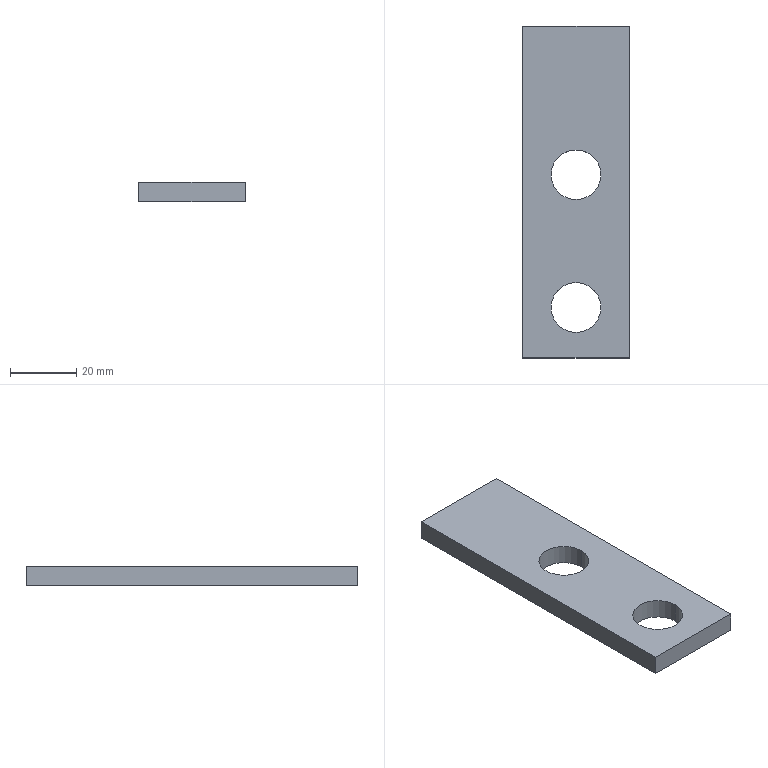Part | SolidWorks | features FlatPattern 1, SMBaseFlange 1, SheetMetal 1 | 1 solid | 10 faces | box 32 x 100 x 6 mm | volume 17079 mm3 | plane 6 | cylinder 4 | commonest cylinder face diameters 15 x4
STEP:
#1=CARTESIAN_POINT('',(8.5,-84.8,-6.));
#2=VERTEX_POINT('',#1);
#3=CARTESIAN_POINT('',(23.5,-84.8,-6.));
#4=VERTEX_POINT('',#3);
#5=CARTESIAN_POINT('',(16.,-84.8,-6.));
#6=DIRECTION('',(0.,0.,1.));
#7=DIRECTION('',(1.,0.,0.));
#8=AXIS2_PLACEMENT_3D('',#5,#6,#7);
#9=CIRCLE('',#8,7.5);
#10=EDGE_CURVE('',#2,#4,#9,.T.);
#11=ORIENTED_EDGE('',*,*,#10,.F.);
#12=CARTESIAN_POINT('',(8.5,-84.8,0.));
#13=VERTEX_POINT('',#12);
#14=CARTESIAN_POINT('',(8.5,-84.8,-6.));
#15=DIRECTION('',(0.,0.,1.));
#16=VECTOR('',#15,1000.);
#17=LINE('',#14,#16);
#18=EDGE_CURVE('',#2,#13,#17,.T.);
#19=ORIENTED_EDGE('',*,*,#18,.T.);
#20=CARTESIAN_POINT('',(23.5,-84.8,0.));
#21=VERTEX_POINT('',#20);
#22=CARTESIAN_POINT('',(16.,-84.8,0.));
#23=DIRECTION('',(0.,0.,1.));
#24=DIRECTION('',(1.,0.,0.));
#25=AXIS2_PLACEMENT_3D('',#22,#23,#24);
#26=CIRCLE('',#25,7.5);
#27=EDGE_CURVE('',#13,#21,#26,.T.);
#28=ORIENTED_EDGE('',*,*,#27,.T.);
#29=CARTESIAN_POINT('',(23.5,-84.8,-6.));
#30=DIRECTION('',(0.,0.,1.));
#31=VECTOR('',#30,1000.);
#32=LINE('',#29,#31);
#33=EDGE_CURVE('',#4,#21,#32,.T.);
#34=ORIENTED_EDGE('',*,*,#33,.F.);
#35=EDGE_LOOP('',(#11,#19,#28,#34));
#36=FACE_OUTER_BOUND('',#35,.T.);
#37=CARTESIAN_POINT('',(16.,-84.8,-6.));
#38=DIRECTION('',(0.,0.,1.));
#39=DIRECTION('',(1.,0.,0.));
#40=AXIS2_PLACEMENT_3D('',#37,#38,#39);
#41=CYLINDRICAL_SURFACE('',#40,7.5);
#42=ADVANCED_FACE('',(#36),#41,.F.);
#43=CARTESIAN_POINT('',(8.5,-44.8,-6.));
#44=VERTEX_POINT('',#43);
#45=CARTESIAN_POINT('',(23.5,-44.8,-6.));
#46=VERTEX_POINT('',#45);
#47=CARTESIAN_POINT('',(16.,-44.8,-6.));
#48=DIRECTION('',(0.,0.,1.));
#49=DIRECTION('',(1.,0.,0.));
#50=AXIS2_PLACEMENT_3D('',#47,#48,#49);
#51=CIRCLE('',#50,7.5);
#52=EDGE_CURVE('',#44,#46,#51,.T.);
#53=ORIENTED_EDGE('',*,*,#52,.F.);
#54=CARTESIAN_POINT('',(8.5,-44.8,0.));
#55=VERTEX_POINT('',#54);
#56=CARTESIAN_POINT('',(8.5,-44.8,-6.));
#57=DIRECTION('',(0.,0.,1.));
#58=VECTOR('',#57,1000.);
#59=LINE('',#56,#58);
#60=EDGE_CURVE('',#44,#55,#59,.T.);
#61=ORIENTED_EDGE('',*,*,#60,.T.);
#62=CARTESIAN_POINT('',(23.5,-44.8,0.));
#63=VERTEX_POINT('',#62);
#64=CARTESIAN_POINT('',(16.,-44.8,0.));
#65=DIRECTION('',(0.,0.,1.));
#66=DIRECTION('',(1.,0.,0.));
#67=AXIS2_PLACEMENT_3D('',#64,#65,#66);
#68=CIRCLE('',#67,7.5);
#69=EDGE_CURVE('',#55,#63,#68,.T.);
#70=ORIENTED_EDGE('',*,*,#69,.T.);
#71=CARTESIAN_POINT('',(23.5,-44.8,-6.));
#72=DIRECTION('',(0.,0.,1.));
#73=VECTOR('',#72,1000.);
#74=LINE('',#71,#73);
#75=EDGE_CURVE('',#46,#63,#74,.T.);
#76=ORIENTED_EDGE('',*,*,#75,.F.);
#77=EDGE_LOOP('',(#53,#61,#70,#76));
#78=FACE_OUTER_BOUND('',#77,.T.);
#79=CARTESIAN_POINT('',(16.,-44.8,-6.));
#80=DIRECTION('',(0.,0.,1.));
#81=DIRECTION('',(1.,0.,0.));
#82=AXIS2_PLACEMENT_3D('',#79,#80,#81);
#83=CYLINDRICAL_SURFACE('',#82,7.5);
#84=ADVANCED_FACE('',(#78),#83,.F.);
#85=CARTESIAN_POINT('',(0.,0.,0.));
#86=VERTEX_POINT('',#85);
#87=CARTESIAN_POINT('',(0.,-100.,0.));
#88=VERTEX_POINT('',#87);
#89=CARTESIAN_POINT('',(0.,0.,0.));
#90=DIRECTION('',(0.,-1.,0.));
#91=VECTOR('',#90,1000.);
#92=LINE('',#89,#91);
#93=EDGE_CURVE('',#86,#88,#92,.T.);
#94=ORIENTED_EDGE('',*,*,#93,.F.);
#95=CARTESIAN_POINT('',(0.,0.,-6.));
#96=VERTEX_POINT('',#95);
#97=CARTESIAN_POINT('',(0.,0.,-6.));
#98=DIRECTION('',(0.,0.,1.));
#99=VECTOR('',#98,1000.);
#100=LINE('',#97,#99);
#101=EDGE_CURVE('',#96,#86,#100,.T.);
#102=ORIENTED_EDGE('',*,*,#101,.F.);
#103=CARTESIAN_POINT('',(0.,-100.,-6.));
#104=VERTEX_POINT('',#103);
#105=CARTESIAN_POINT('',(0.,0.,-6.));
#106=DIRECTION('',(0.,-1.,0.));
#107=VECTOR('',#106,1000.);
#108=LINE('',#105,#107);
#109=EDGE_CURVE('',#96,#104,#108,.T.);
#110=ORIENTED_EDGE('',*,*,#109,.T.);
#111=CARTESIAN_POINT('',(0.,-100.,-6.));
#112=DIRECTION('',(0.,0.,1.));
#113=VECTOR('',#112,1000.);
#114=LINE('',#111,#113);
#115=EDGE_CURVE('',#104,#88,#114,.T.);
#116=ORIENTED_EDGE('',*,*,#115,.T.);
#117=EDGE_LOOP('',(#94,#102,#110,#116));
#118=FACE_OUTER_BOUND('',#117,.T.);
#119=CARTESIAN_POINT('',(0.,0.,-6.));
#120=DIRECTION('',(-1.,0.,0.));
#121=DIRECTION('',(0.,-1.,0.));
#122=AXIS2_PLACEMENT_3D('',#119,#120,#121);
#123=PLANE('',#122);
#124=ADVANCED_FACE('',(#118),#123,.T.);
#125=CARTESIAN_POINT('',(32.,0.,0.));
#126=VERTEX_POINT('',#125);
#127=CARTESIAN_POINT('',(0.,0.,0.));
#128=DIRECTION('',(-1.,0.,0.));
#129=VECTOR('',#128,1000.);
#130=LINE('',#127,#129);
#131=EDGE_CURVE('',#126,#86,#130,.T.);
#132=ORIENTED_EDGE('',*,*,#131,.F.);
#133=CARTESIAN_POINT('',(32.,0.,-6.));
#134=VERTEX_POINT('',#133);
#135=CARTESIAN_POINT('',(32.,0.,-6.));
#136=DIRECTION('',(0.,0.,1.));
#137=VECTOR('',#136,1000.);
#138=LINE('',#135,#137);
#139=EDGE_CURVE('',#134,#126,#138,.T.);
#140=ORIENTED_EDGE('',*,*,#139,.F.);
#141=CARTESIAN_POINT('',(0.,0.,-6.));
#142=DIRECTION('',(-1.,0.,0.));
#143=VECTOR('',#142,1000.);
#144=LINE('',#141,#143);
#145=EDGE_CURVE('',#134,#96,#144,.T.);
#146=ORIENTED_EDGE('',*,*,#145,.T.);
#147=ORIENTED_EDGE('',*,*,#101,.T.);
#148=EDGE_LOOP('',(#132,#140,#146,#147));
#149=FACE_OUTER_BOUND('',#148,.T.);
#150=CARTESIAN_POINT('',(0.,0.,-6.));
#151=DIRECTION('',(0.,1.,0.));
#152=DIRECTION('',(0.,0.,1.));
#153=AXIS2_PLACEMENT_3D('',#150,#151,#152);
#154=PLANE('',#153);
#155=ADVANCED_FACE('',(#149),#154,.T.);
#156=CARTESIAN_POINT('',(32.,-100.,0.));
#157=VERTEX_POINT('',#156);
#158=CARTESIAN_POINT('',(32.,0.,0.));
#159=DIRECTION('',(0.,1.,0.));
#160=VECTOR('',#159,1000.);
#161=LINE('',#158,#160);
#162=EDGE_CURVE('',#157,#126,#161,.T.);
#163=ORIENTED_EDGE('',*,*,#162,.F.);
#164=CARTESIAN_POINT('',(32.,-100.,-6.));
#165=VERTEX_POINT('',#164);
#166=CARTESIAN_POINT('',(32.,-100.,-6.));
#167=DIRECTION('',(0.,0.,1.));
#168=VECTOR('',#167,1000.);
#169=LINE('',#166,#168);
#170=EDGE_CURVE('',#165,#157,#169,.T.);
#171=ORIENTED_EDGE('',*,*,#170,.F.);
#172=CARTESIAN_POINT('',(32.,0.,-6.));
#173=DIRECTION('',(0.,1.,0.));
#174=VECTOR('',#173,1000.);
#175=LINE('',#172,#174);
#176=EDGE_CURVE('',#165,#134,#175,.T.);
#177=ORIENTED_EDGE('',*,*,#176,.T.);
#178=ORIENTED_EDGE('',*,*,#139,.T.);
#179=EDGE_LOOP('',(#163,#171,#177,#178));
#180=FACE_OUTER_BOUND('',#179,.T.);
#181=CARTESIAN_POINT('',(32.,0.,-6.));
#182=DIRECTION('',(1.,0.,0.));
#183=DIRECTION('',(0.,1.,0.));
#184=AXIS2_PLACEMENT_3D('',#181,#182,#183);
#185=PLANE('',#184);
#186=ADVANCED_FACE('',(#180),#185,.T.);
#187=CARTESIAN_POINT('',(0.,-100.,0.));
#188=DIRECTION('',(1.,0.,0.));
#189=VECTOR('',#188,1000.);
#190=LINE('',#187,#189);
#191=EDGE_CURVE('',#88,#157,#190,.T.);
#192=ORIENTED_EDGE('',*,*,#191,.F.);
#193=ORIENTED_EDGE('',*,*,#115,.F.);
#194=CARTESIAN_POINT('',(0.,-100.,-6.));
#195=DIRECTION('',(1.,0.,0.));
#196=VECTOR('',#195,1000.);
#197=LINE('',#194,#196);
#198=EDGE_CURVE('',#104,#165,#197,.T.);
#199=ORIENTED_EDGE('',*,*,#198,.T.);
#200=ORIENTED_EDGE('',*,*,#170,.T.);
#201=EDGE_LOOP('',(#192,#193,#199,#200));
#202=FACE_OUTER_BOUND('',#201,.T.);
#203=CARTESIAN_POINT('',(0.,-100.,-6.));
#204=DIRECTION('',(0.,-1.,0.));
#205=DIRECTION('',(0.,0.,-1.));
#206=AXIS2_PLACEMENT_3D('',#203,#204,#205);
#207=PLANE('',#206);
#208=ADVANCED_FACE('',(#202),#207,.T.);
#209=CARTESIAN_POINT('',(16.,-84.8,-6.));
#210=DIRECTION('',(0.,0.,1.));
#211=DIRECTION('',(1.,0.,0.));
#212=AXIS2_PLACEMENT_3D('',#209,#210,#211);
#213=CIRCLE('',#212,7.5);
#214=EDGE_CURVE('',#4,#2,#213,.T.);
#215=ORIENTED_EDGE('',*,*,#214,.T.);
#216=ORIENTED_EDGE('',*,*,#10,.T.);
#217=EDGE_LOOP('',(#215,#216));
#218=FACE_BOUND('',#217,.T.);
#219=CARTESIAN_POINT('',(16.,-44.8,-6.));
#220=DIRECTION('',(0.,0.,1.));
#221=DIRECTION('',(1.,0.,0.));
#222=AXIS2_PLACEMENT_3D('',#219,#220,#221);
#223=CIRCLE('',#222,7.5);
#224=EDGE_CURVE('',#46,#44,#223,.T.);
#225=ORIENTED_EDGE('',*,*,#224,.T.);
#226=ORIENTED_EDGE('',*,*,#52,.T.);
#227=EDGE_LOOP('',(#225,#226));
#228=FACE_BOUND('',#227,.T.);
#229=ORIENTED_EDGE('',*,*,#109,.F.);
#230=ORIENTED_EDGE('',*,*,#145,.F.);
#231=ORIENTED_EDGE('',*,*,#176,.F.);
#232=ORIENTED_EDGE('',*,*,#198,.F.);
#233=EDGE_LOOP('',(#229,#230,#231,#232));
#234=FACE_OUTER_BOUND('',#233,.T.);
#235=CARTESIAN_POINT('',(0.,0.,-6.));
#236=DIRECTION('',(0.,0.,1.));
#237=DIRECTION('',(1.,0.,0.));
#238=AXIS2_PLACEMENT_3D('',#235,#236,#237);
#239=PLANE('',#238);
#240=ADVANCED_FACE('',(#218,#228,#234),#239,.F.);
#241=CARTESIAN_POINT('',(16.,-84.8,0.));
#242=DIRECTION('',(0.,0.,1.));
#243=DIRECTION('',(1.,0.,0.));
#244=AXIS2_PLACEMENT_3D('',#241,#242,#243);
#245=CIRCLE('',#244,7.5);
#246=EDGE_CURVE('',#21,#13,#245,.T.);
#247=ORIENTED_EDGE('',*,*,#246,.F.);
#248=ORIENTED_EDGE('',*,*,#27,.F.);
#249=EDGE_LOOP('',(#247,#248));
#250=FACE_BOUND('',#249,.T.);
#251=CARTESIAN_POINT('',(16.,-44.8,0.));
#252=DIRECTION('',(0.,0.,1.));
#253=DIRECTION('',(1.,0.,0.));
#254=AXIS2_PLACEMENT_3D('',#251,#252,#253);
#255=CIRCLE('',#254,7.5);
#256=EDGE_CURVE('',#63,#55,#255,.T.);
#257=ORIENTED_EDGE('',*,*,#256,.F.);
#258=ORIENTED_EDGE('',*,*,#69,.F.);
#259=EDGE_LOOP('',(#257,#258));
#260=FACE_BOUND('',#259,.T.);
#261=ORIENTED_EDGE('',*,*,#93,.T.);
#262=ORIENTED_EDGE('',*,*,#191,.T.);
#263=ORIENTED_EDGE('',*,*,#162,.T.);
#264=ORIENTED_EDGE('',*,*,#131,.T.);
#265=EDGE_LOOP('',(#261,#262,#263,#264));
#266=FACE_OUTER_BOUND('',#265,.T.);
#267=CARTESIAN_POINT('',(0.,0.,0.));
#268=DIRECTION('',(0.,0.,1.));
#269=DIRECTION('',(1.,0.,0.));
#270=AXIS2_PLACEMENT_3D('',#267,#268,#269);
#271=PLANE('',#270);
#272=ADVANCED_FACE('',(#250,#260,#266),#271,.T.);
#273=ORIENTED_EDGE('',*,*,#60,.F.);
#274=ORIENTED_EDGE('',*,*,#224,.F.);
#275=ORIENTED_EDGE('',*,*,#75,.T.);
#276=ORIENTED_EDGE('',*,*,#256,.T.);
#277=EDGE_LOOP('',(#273,#274,#275,#276));
#278=FACE_OUTER_BOUND('',#277,.T.);
#279=CARTESIAN_POINT('',(16.,-44.8,-6.));
#280=DIRECTION('',(0.,0.,1.));
#281=DIRECTION('',(1.,0.,0.));
#282=AXIS2_PLACEMENT_3D('',#279,#280,#281);
#283=CYLINDRICAL_SURFACE('',#282,7.5);
#284=ADVANCED_FACE('',(#278),#283,.F.);
#285=ORIENTED_EDGE('',*,*,#18,.F.);
#286=ORIENTED_EDGE('',*,*,#214,.F.);
#287=ORIENTED_EDGE('',*,*,#33,.T.);
#288=ORIENTED_EDGE('',*,*,#246,.T.);
#289=EDGE_LOOP('',(#285,#286,#287,#288));
#290=FACE_OUTER_BOUND('',#289,.T.);
#291=CARTESIAN_POINT('',(16.,-84.8,-6.));
#292=DIRECTION('',(0.,0.,1.));
#293=DIRECTION('',(1.,0.,0.));
#294=AXIS2_PLACEMENT_3D('',#291,#292,#293);
#295=CYLINDRICAL_SURFACE('',#294,7.5);
#296=ADVANCED_FACE('',(#290),#295,.F.);
#297=CLOSED_SHELL('',(#42,#84,#124,#155,#186,#208,#240,#272,#284,#296));
#298=MANIFOLD_SOLID_BREP('',#297);
#299=CARTESIAN_POINT('',(0.,0.,0.));
#300=DIRECTION('',(0.,0.,1.));
#301=DIRECTION('',(1.,0.,0.));
#302=AXIS2_PLACEMENT_3D('',#299,#300,#301);
#303=(LENGTH_UNIT()NAMED_UNIT(*)SI_UNIT(.MILLI.,.METRE.));
#304=UNCERTAINTY_MEASURE_WITH_UNIT(LENGTH_MEASURE(0.00001),#303,'','');
#305=(NAMED_UNIT(*)PLANE_ANGLE_UNIT()SI_UNIT($,.RADIAN.));
#306=(NAMED_UNIT(*)SI_UNIT($,.STERADIAN.)SOLID_ANGLE_UNIT());
#307=(GEOMETRIC_REPRESENTATION_CONTEXT(3)GLOBAL_UNCERTAINTY_ASSIGNED_CONTEXT((#304))GLOBAL_UNIT_ASSIGNED_CONTEXT((#303,#305,#306))REPRESENTATION_CONTEXT('',''));
#308=ADVANCED_BREP_SHAPE_REPRESENTATION('',(#298,#302),#307);